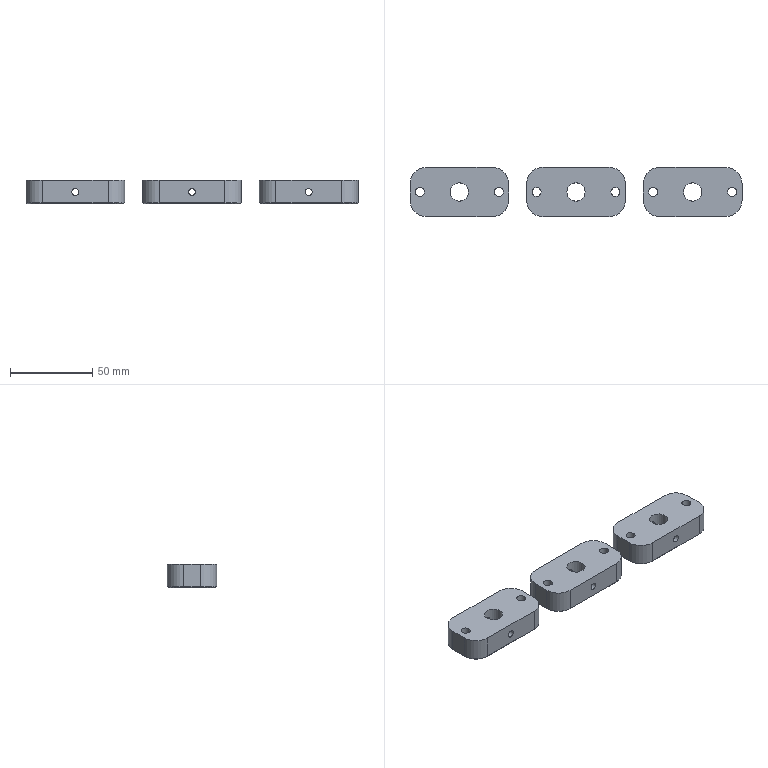CAM job | NX | 3-axis milling, drilling | part box 202 x 30 x 14 mm | stock box 207 x 35 x 20 mm
Tools:
number,name,description,diameter,corner_radius,flute_length,length,flutes
4,D4,平底铣刀-粗,4.0,0.0,25.0,75.0,2
6,D6,平底铣刀-粗,6.0,0.0,25.0,75.0,2
9,D10,平底铣刀-粗,10.0,0.0,35.0,75.0,2
7,D6-J,平底铣刀-精,6.0,0.0,25.0,75.0,2
10,D10-J,平底铣刀-精,10.0,0.0,35.0,75.0,2
1,D80R0.8飞刀,圆鼻刀-粗,80.0,0.8,50.0,75.0,2
1,D80R0.8飞刀-J,圆鼻刀-精,80.0,0.8,50.0,75.0,2
2,D6倒角刀,倒角刀,6.0,0.0,3.0,25.0,2
17,ZT5.5,钻头,5.5,0.0,35.0,50.0,2
17,钻头5.5,Twist Drill 5 mm,5.5,0.0,52.0,54.0,2
Operations:
program,operation,operation_type,tool,method,geometry_group,spindle_rpm,surface_speed,feed_per_tooth,feed_cut,feed_plunge,cut_length_mm,path_length_mm,cut_time_min,machine_time_min
B,FLOOR_WALL_FLY_FACE_ROUGH_COPY,VolumeBased25DMillingOperation,D80R0.8飞刀,LAYER_ROUGH-DEPTHK-STEPG,W-B,2800.0,703.696,0.5357,3000.0,100.0,3722.328,7377.038,1.241,1.606
B,FLOOR_WALL_FLY_FACE_FINISH_COPY,VolumeBased25DMillingOperation,D80R0.8飞刀-J,SIDE_FINISH-DEPTHK-STEPG,W-B,4000.0,1005.28,0.125,1000.0,100.0,309.998,345.998,0.31,0.3136
B,C0.3_PLANAR_DEBURR_6X45L__COPY,SurfaceContour,D6倒角刀,CLIMB_FACE_CHAMFER-DEPTH0-STEPG,W-B,8000.0,150.796,0.0938,1500.0,90.0,710.088,1385.291,0.4752,0.5427
A,TOP_FACE,FaceMilling,D80R0.8飞刀,SIDE_FINISH-DEPTHK-STEPG,W-A,5000.0,1256.637,0.1,1000.0,100.0,296.0,332.0,0.296,0.2996
A,PROFILE_ROUGH_2,VolumeBased25DMillingOperation,D10,METHOD,W-A,8000.0,251.327,0.3125,5000.0,80.0,11697.157,12069.157,2.339,2.377
A,SPOT_0.8,Operation,D6倒角刀,METHOD,W-A,8000.0,150.796,0.0312,500.0,0.0,5.4,194.814,0.0108,0.0297
A,COUNTERSINK_SPOT-DEPTH0.8,Operation,D6倒角刀,NONE,W-A,8000.0,150.796,0.0312,500.0,90.0,10.8,256.675,0.0216,0.0462
A,COUNTERSINK_DRILL_SEG0,Operation,钻头5.5,NONE,W-A,2800.0,48.38,0.0357,200.0,90.0,111.914,458.903,0.5596,0.5943
A,THROUGH_HOLE-10-12.5,Operation,ZT5.5,NONE,W-A,1500.0,52.119,0.1,300.0,90.0,69.0,322.014,0.23,0.2553
A,FLOOR_WALL_HELICAL_ROUGH-MID_COPY,VolumeBased25DMillingOperation,D6,LAYER_ROUGH-DEPTHK-STEPG,W-A,8000.0,150.796,0.125,2000.0,100.0,2352.164,2652.542,1.176,1.206
A,HOLE_MILL_ROUGH_D4_1,CylinderMilling,D4,NONE,W-A,8000.0,100.531,0.075,1200.0,100.0,3145.269,3641.269,2.621,2.671
A,HOLE_MILL_FINISH_D4_1,CylinderMilling,D4,FINISH_STEP_DEPTH_OFF,W-A,8000.0,100.531,0.0312,500.0,100.0,269.67,726.67,0.5393,0.585
A,MILL_CHAMFER_1,PlanarMilling,D6倒角刀,NONE,W-A,8000.0,150.796,0.0312,500.0,100.0,220.118,594.31,0.4402,0.4777
A,MILL_CHAMFER_2,PlanarMilling,D6倒角刀,METHOD,W-A,8000.0,150.796,0.05,800.0,100.0,122.318,387.824,0.1529,0.1794
A,FLOOR_WALL_CHAMFER_COPY,VolumeBased25DMillingOperation,D6倒角刀,CLIMB_FACE_CHAMFER-DEPTH0-STEPG,W-A,6500.0,122.519,0.1154,1500.0,100.0,523.079,750.673,0.3487,0.3715
A,FLOOR_WALL_FINISH_SIDE-MID_COPY,VolumeBased25DMillingOperation,D6-J,SIDE_FINISH-DEPTHK-STEPG,W-A,8000.0,150.796,0.0375,600.0,100.0,139.102,417.549,0.2318,0.2597
A,PROFILE_SEMI-FINISH_2,VolumeBased25DMillingOperation,D10-J,METHOD,W-A,8000.0,251.327,0.0625,1000.0,100.0,597.837,958.837,0.5978,0.6339